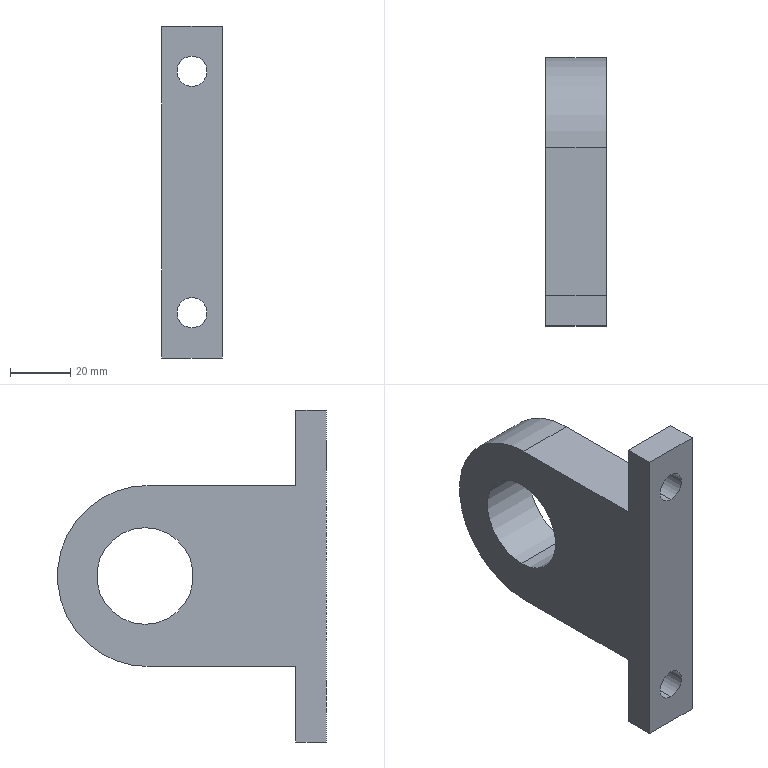Part | SolidWorks | features MoveFace 4, BaseBody 1, DelFace 1, HoleWzd 1, ICE 1, Split 1 | 1 solid | 16 faces | box 20 x 89 x 110 mm | volume 91419 mm3 | plane 9 | cylinder 7 | commonest cylinder face diameters 10 x4 32 x2 60 x1
STEP:
#1=CARTESIAN_POINT('',(-25.,46.,-25.));
#2=VERTEX_POINT('',#1);
#3=CARTESIAN_POINT('',(-25.,46.,-15.));
#4=VERTEX_POINT('',#3);
#5=CARTESIAN_POINT('',(-25.,46.,-20.));
#6=DIRECTION('',(0.,1.,0.));
#7=DIRECTION('',(-1.,0.,0.));
#8=AXIS2_PLACEMENT_3D('',#5,#6,#7);
#9=CIRCLE('',#8,5.);
#10=EDGE_CURVE('',#2,#4,#9,.T.);
#11=ORIENTED_EDGE('',*,*,#10,.F.);
#12=CARTESIAN_POINT('',(-25.,56.,-25.));
#13=VERTEX_POINT('',#12);
#14=CARTESIAN_POINT('',(-25.,10.,-25.));
#15=DIRECTION('',(0.,1.,0.));
#16=VECTOR('',#15,1000.);
#17=LINE('',#14,#16);
#18=EDGE_CURVE('',#2,#13,#17,.T.);
#19=ORIENTED_EDGE('',*,*,#18,.T.);
#20=CARTESIAN_POINT('',(-25.,56.,-15.));
#21=VERTEX_POINT('',#20);
#22=CARTESIAN_POINT('',(-25.,56.,-20.));
#23=DIRECTION('',(0.,1.,0.));
#24=DIRECTION('',(-1.,0.,0.));
#25=AXIS2_PLACEMENT_3D('',#22,#23,#24);
#26=CIRCLE('',#25,5.);
#27=EDGE_CURVE('',#13,#21,#26,.T.);
#28=ORIENTED_EDGE('',*,*,#27,.T.);
#29=CARTESIAN_POINT('',(-25.,10.,-15.));
#30=DIRECTION('',(0.,1.,0.));
#31=VECTOR('',#30,1000.);
#32=LINE('',#29,#31);
#33=EDGE_CURVE('',#4,#21,#32,.T.);
#34=ORIENTED_EDGE('',*,*,#33,.F.);
#35=EDGE_LOOP('',(#11,#19,#28,#34));
#36=FACE_OUTER_BOUND('',#35,.T.);
#37=CARTESIAN_POINT('',(-25.,10.,-20.));
#38=DIRECTION('',(0.,1.,0.));
#39=DIRECTION('',(0.,0.,1.));
#40=AXIS2_PLACEMENT_3D('',#37,#38,#39);
#41=CYLINDRICAL_SURFACE('',#40,5.);
#42=ADVANCED_FACE('',(#36),#41,.F.);
#43=CARTESIAN_POINT('',(-25.,46.,55.));
#44=VERTEX_POINT('',#43);
#45=CARTESIAN_POINT('',(-25.,46.,65.));
#46=VERTEX_POINT('',#45);
#47=CARTESIAN_POINT('',(-25.,46.,60.));
#48=DIRECTION('',(0.,1.,0.));
#49=DIRECTION('',(-1.,0.,0.));
#50=AXIS2_PLACEMENT_3D('',#47,#48,#49);
#51=CIRCLE('',#50,5.);
#52=EDGE_CURVE('',#44,#46,#51,.T.);
#53=ORIENTED_EDGE('',*,*,#52,.F.);
#54=CARTESIAN_POINT('',(-25.,56.,55.));
#55=VERTEX_POINT('',#54);
#56=CARTESIAN_POINT('',(-25.,10.,55.));
#57=DIRECTION('',(0.,1.,0.));
#58=VECTOR('',#57,1000.);
#59=LINE('',#56,#58);
#60=EDGE_CURVE('',#44,#55,#59,.T.);
#61=ORIENTED_EDGE('',*,*,#60,.T.);
#62=CARTESIAN_POINT('',(-25.,56.,65.));
#63=VERTEX_POINT('',#62);
#64=CARTESIAN_POINT('',(-25.,56.,60.));
#65=DIRECTION('',(0.,1.,0.));
#66=DIRECTION('',(-1.,0.,0.));
#67=AXIS2_PLACEMENT_3D('',#64,#65,#66);
#68=CIRCLE('',#67,5.);
#69=EDGE_CURVE('',#55,#63,#68,.T.);
#70=ORIENTED_EDGE('',*,*,#69,.T.);
#71=CARTESIAN_POINT('',(-25.,10.,65.));
#72=DIRECTION('',(0.,1.,0.));
#73=VECTOR('',#72,1000.);
#74=LINE('',#71,#73);
#75=EDGE_CURVE('',#46,#63,#74,.T.);
#76=ORIENTED_EDGE('',*,*,#75,.F.);
#77=EDGE_LOOP('',(#53,#61,#70,#76));
#78=FACE_OUTER_BOUND('',#77,.T.);
#79=CARTESIAN_POINT('',(-25.,10.,60.));
#80=DIRECTION('',(0.,1.,0.));
#81=DIRECTION('',(0.,0.,1.));
#82=AXIS2_PLACEMENT_3D('',#79,#80,#81);
#83=CYLINDRICAL_SURFACE('',#82,5.);
#84=ADVANCED_FACE('',(#78),#83,.F.);
#85=CARTESIAN_POINT('',(-35.,106.,36.));
#86=VERTEX_POINT('',#85);
#87=CARTESIAN_POINT('',(-35.,106.,4.));
#88=VERTEX_POINT('',#87);
#89=CARTESIAN_POINT('',(-35.,106.,20.));
#90=DIRECTION('',(1.,0.,0.));
#91=DIRECTION('',(0.,0.,-1.));
#92=AXIS2_PLACEMENT_3D('',#89,#90,#91);
#93=CIRCLE('',#92,16.);
#94=EDGE_CURVE('',#86,#88,#93,.T.);
#95=ORIENTED_EDGE('',*,*,#94,.F.);
#96=CARTESIAN_POINT('',(-15.,106.,36.));
#97=VERTEX_POINT('',#96);
#98=CARTESIAN_POINT('',(-35.,106.,36.));
#99=DIRECTION('',(1.,0.,0.));
#100=VECTOR('',#99,1000.);
#101=LINE('',#98,#100);
#102=EDGE_CURVE('',#86,#97,#101,.T.);
#103=ORIENTED_EDGE('',*,*,#102,.T.);
#104=CARTESIAN_POINT('',(-15.,106.,4.));
#105=VERTEX_POINT('',#104);
#106=CARTESIAN_POINT('',(-15.,106.,20.));
#107=DIRECTION('',(-1.,0.,0.));
#108=DIRECTION('',(0.,-1.,0.));
#109=AXIS2_PLACEMENT_3D('',#106,#107,#108);
#110=CIRCLE('',#109,16.);
#111=EDGE_CURVE('',#105,#97,#110,.T.);
#112=ORIENTED_EDGE('',*,*,#111,.F.);
#113=CARTESIAN_POINT('',(-35.,106.,4.));
#114=DIRECTION('',(1.,0.,0.));
#115=VECTOR('',#114,1000.);
#116=LINE('',#113,#115);
#117=EDGE_CURVE('',#88,#105,#116,.T.);
#118=ORIENTED_EDGE('',*,*,#117,.F.);
#119=EDGE_LOOP('',(#95,#103,#112,#118));
#120=FACE_OUTER_BOUND('',#119,.T.);
#121=CARTESIAN_POINT('',(-35.,106.,20.));
#122=DIRECTION('',(1.,0.,0.));
#123=DIRECTION('',(0.,0.,-1.));
#124=AXIS2_PLACEMENT_3D('',#121,#122,#123);
#125=CYLINDRICAL_SURFACE('',#124,16.);
#126=ADVANCED_FACE('',(#120),#125,.F.);
#127=CARTESIAN_POINT('',(-25.,46.,-20.));
#128=DIRECTION('',(0.,1.,0.));
#129=DIRECTION('',(-1.,0.,0.));
#130=AXIS2_PLACEMENT_3D('',#127,#128,#129);
#131=CIRCLE('',#130,5.);
#132=EDGE_CURVE('',#4,#2,#131,.T.);
#133=ORIENTED_EDGE('',*,*,#132,.T.);
#134=ORIENTED_EDGE('',*,*,#10,.T.);
#135=EDGE_LOOP('',(#133,#134));
#136=FACE_BOUND('',#135,.T.);
#137=CARTESIAN_POINT('',(-25.,46.,60.));
#138=DIRECTION('',(0.,1.,0.));
#139=DIRECTION('',(-1.,0.,0.));
#140=AXIS2_PLACEMENT_3D('',#137,#138,#139);
#141=CIRCLE('',#140,5.);
#142=EDGE_CURVE('',#46,#44,#141,.T.);
#143=ORIENTED_EDGE('',*,*,#142,.T.);
#144=ORIENTED_EDGE('',*,*,#52,.T.);
#145=EDGE_LOOP('',(#143,#144));
#146=FACE_BOUND('',#145,.T.);
#147=CARTESIAN_POINT('',(-15.,46.,75.));
#148=VERTEX_POINT('',#147);
#149=CARTESIAN_POINT('',(-15.,46.,-35.));
#150=VERTEX_POINT('',#149);
#151=CARTESIAN_POINT('',(-15.,46.,40.));
#152=DIRECTION('',(0.,0.,-1.));
#153=VECTOR('',#152,1000.);
#154=LINE('',#151,#153);
#155=EDGE_CURVE('',#148,#150,#154,.T.);
#156=ORIENTED_EDGE('',*,*,#155,.F.);
#157=CARTESIAN_POINT('',(-35.,46.,75.));
#158=VERTEX_POINT('',#157);
#159=CARTESIAN_POINT('',(-35.,46.,75.));
#160=DIRECTION('',(-1.,0.,0.));
#161=VECTOR('',#160,1000.);
#162=LINE('',#159,#161);
#163=EDGE_CURVE('',#148,#158,#162,.T.);
#164=ORIENTED_EDGE('',*,*,#163,.T.);
#165=CARTESIAN_POINT('',(-35.,46.,-35.));
#166=VERTEX_POINT('',#165);
#167=CARTESIAN_POINT('',(-35.,46.,40.));
#168=DIRECTION('',(0.,0.,-1.));
#169=VECTOR('',#168,1000.);
#170=LINE('',#167,#169);
#171=EDGE_CURVE('',#158,#166,#170,.T.);
#172=ORIENTED_EDGE('',*,*,#171,.T.);
#173=CARTESIAN_POINT('',(-35.,46.,-35.));
#174=DIRECTION('',(1.,0.,0.));
#175=VECTOR('',#174,1000.);
#176=LINE('',#173,#175);
#177=EDGE_CURVE('',#166,#150,#176,.T.);
#178=ORIENTED_EDGE('',*,*,#177,.T.);
#179=EDGE_LOOP('',(#156,#164,#172,#178));
#180=FACE_OUTER_BOUND('',#179,.T.);
#181=CARTESIAN_POINT('',(0.,46.,40.));
#182=DIRECTION('',(0.,1.,0.));
#183=DIRECTION('',(-1.,0.,0.));
#184=AXIS2_PLACEMENT_3D('',#181,#182,#183);
#185=PLANE('',#184);
#186=ADVANCED_FACE('',(#136,#146,#180),#185,.F.);
#187=CARTESIAN_POINT('',(-35.,105.,50.));
#188=VERTEX_POINT('',#187);
#189=CARTESIAN_POINT('',(-35.,56.,50.));
#190=VERTEX_POINT('',#189);
#191=CARTESIAN_POINT('',(-35.,0.,50.));
#192=DIRECTION('',(0.,-1.,0.));
#193=VECTOR('',#192,1000.);
#194=LINE('',#191,#193);
#195=EDGE_CURVE('',#188,#190,#194,.T.);
#196=ORIENTED_EDGE('',*,*,#195,.T.);
#197=CARTESIAN_POINT('',(-15.,56.,50.));
#198=VERTEX_POINT('',#197);
#199=CARTESIAN_POINT('',(0.,56.,50.));
#200=DIRECTION('',(1.,0.,0.));
#201=VECTOR('',#200,1000.);
#202=LINE('',#199,#201);
#203=EDGE_CURVE('',#190,#198,#202,.T.);
#204=ORIENTED_EDGE('',*,*,#203,.T.);
#205=CARTESIAN_POINT('',(-15.,105.,50.));
#206=VERTEX_POINT('',#205);
#207=CARTESIAN_POINT('',(-15.,125.,50.));
#208=DIRECTION('',(0.,-1.,0.));
#209=VECTOR('',#208,1000.);
#210=LINE('',#207,#209);
#211=EDGE_CURVE('',#206,#198,#210,.T.);
#212=ORIENTED_EDGE('',*,*,#211,.F.);
#213=CARTESIAN_POINT('',(0.,105.,50.));
#214=DIRECTION('',(1.,0.,0.));
#215=VECTOR('',#214,1000.);
#216=LINE('',#213,#215);
#217=EDGE_CURVE('',#188,#206,#216,.T.);
#218=ORIENTED_EDGE('',*,*,#217,.F.);
#219=EDGE_LOOP('',(#196,#204,#212,#218));
#220=FACE_OUTER_BOUND('',#219,.T.);
#221=CARTESIAN_POINT('',(0.,0.,50.));
#222=DIRECTION('',(0.,0.,-1.));
#223=DIRECTION('',(-1.,0.,0.));
#224=AXIS2_PLACEMENT_3D('',#221,#222,#223);
#225=PLANE('',#224);
#226=ADVANCED_FACE('',(#220),#225,.F.);
#227=CARTESIAN_POINT('',(-35.,56.,-10.));
#228=VERTEX_POINT('',#227);
#229=CARTESIAN_POINT('',(-35.,105.,-10.));
#230=VERTEX_POINT('',#229);
#231=CARTESIAN_POINT('',(-35.,0.,-10.));
#232=DIRECTION('',(0.,1.,0.));
#233=VECTOR('',#232,1000.);
#234=LINE('',#231,#233);
#235=EDGE_CURVE('',#228,#230,#234,.T.);
#236=ORIENTED_EDGE('',*,*,#235,.F.);
#237=CARTESIAN_POINT('',(-35.,56.,-35.));
#238=VERTEX_POINT('',#237);
#239=CARTESIAN_POINT('',(-35.,56.,0.));
#240=DIRECTION('',(0.,0.,-1.));
#241=VECTOR('',#240,1000.);
#242=LINE('',#239,#241);
#243=EDGE_CURVE('',#228,#238,#242,.T.);
#244=ORIENTED_EDGE('',*,*,#243,.T.);
#245=CARTESIAN_POINT('',(-35.,10.,-35.));
#246=DIRECTION('',(0.,-1.,0.));
#247=VECTOR('',#246,1000.);
#248=LINE('',#245,#247);
#249=EDGE_CURVE('',#238,#166,#248,.T.);
#250=ORIENTED_EDGE('',*,*,#249,.T.);
#251=ORIENTED_EDGE('',*,*,#171,.F.);
#252=CARTESIAN_POINT('',(-35.,56.,75.));
#253=VERTEX_POINT('',#252);
#254=CARTESIAN_POINT('',(-35.,10.,75.));
#255=DIRECTION('',(0.,-1.,0.));
#256=VECTOR('',#255,1000.);
#257=LINE('',#254,#256);
#258=EDGE_CURVE('',#253,#158,#257,.T.);
#259=ORIENTED_EDGE('',*,*,#258,.F.);
#260=CARTESIAN_POINT('',(-35.,56.,0.));
#261=DIRECTION('',(0.,0.,-1.));
#262=VECTOR('',#261,1000.);
#263=LINE('',#260,#262);
#264=EDGE_CURVE('',#253,#190,#263,.T.);
#265=ORIENTED_EDGE('',*,*,#264,.T.);
#266=ORIENTED_EDGE('',*,*,#195,.F.);
#267=CARTESIAN_POINT('',(-35.,105.,20.));
#268=DIRECTION('',(1.,0.,0.));
#269=DIRECTION('',(0.,0.,-1.));
#270=AXIS2_PLACEMENT_3D('',#267,#268,#269);
#271=CIRCLE('',#270,30.);
#272=EDGE_CURVE('',#230,#188,#271,.T.);
#273=ORIENTED_EDGE('',*,*,#272,.F.);
#274=EDGE_LOOP('',(#236,#244,#250,#251,#259,#265,#266,#273));
#275=FACE_OUTER_BOUND('',#274,.T.);
#276=CARTESIAN_POINT('',(-35.,106.,20.));
#277=DIRECTION('',(1.,0.,0.));
#278=DIRECTION('',(0.,0.,-1.));
#279=AXIS2_PLACEMENT_3D('',#276,#277,#278);
#280=CIRCLE('',#279,16.);
#281=EDGE_CURVE('',#88,#86,#280,.T.);
#282=ORIENTED_EDGE('',*,*,#281,.T.);
#283=ORIENTED_EDGE('',*,*,#94,.T.);
#284=EDGE_LOOP('',(#282,#283));
#285=FACE_BOUND('',#284,.T.);
#286=CARTESIAN_POINT('',(-35.,0.,40.));
#287=DIRECTION('',(1.,0.,0.));
#288=DIRECTION('',(0.,0.,-1.));
#289=AXIS2_PLACEMENT_3D('',#286,#287,#288);
#290=PLANE('',#289);
#291=ADVANCED_FACE('',(#275,#285),#290,.F.);
#292=ORIENTED_EDGE('',*,*,#102,.F.);
#293=ORIENTED_EDGE('',*,*,#281,.F.);
#294=ORIENTED_EDGE('',*,*,#117,.T.);
#295=CARTESIAN_POINT('',(-15.,106.,20.));
#296=DIRECTION('',(-1.,0.,0.));
#297=DIRECTION('',(0.,-1.,0.));
#298=AXIS2_PLACEMENT_3D('',#295,#296,#297);
#299=CIRCLE('',#298,16.);
#300=EDGE_CURVE('',#97,#105,#299,.T.);
#301=ORIENTED_EDGE('',*,*,#300,.F.);
#302=EDGE_LOOP('',(#292,#293,#294,#301));
#303=FACE_OUTER_BOUND('',#302,.T.);
#304=CARTESIAN_POINT('',(-35.,106.,20.));
#305=DIRECTION('',(1.,0.,0.));
#306=DIRECTION('',(0.,0.,-1.));
#307=AXIS2_PLACEMENT_3D('',#304,#305,#306);
#308=CYLINDRICAL_SURFACE('',#307,16.);
#309=ADVANCED_FACE('',(#303),#308,.F.);
#310=CARTESIAN_POINT('',(-15.,56.,-10.));
#311=VERTEX_POINT('',#310);
#312=CARTESIAN_POINT('',(0.,56.,-10.));
#313=DIRECTION('',(1.,0.,0.));
#314=VECTOR('',#313,1000.);
#315=LINE('',#312,#314);
#316=EDGE_CURVE('',#228,#311,#315,.T.);
#317=ORIENTED_EDGE('',*,*,#316,.F.);
#318=ORIENTED_EDGE('',*,*,#235,.T.);
#319=CARTESIAN_POINT('',(-15.,105.,-10.));
#320=VERTEX_POINT('',#319);
#321=CARTESIAN_POINT('',(0.,105.,-10.));
#322=DIRECTION('',(-1.,0.,0.));
#323=VECTOR('',#322,1000.);
#324=LINE('',#321,#323);
#325=EDGE_CURVE('',#320,#230,#324,.T.);
#326=ORIENTED_EDGE('',*,*,#325,.F.);
#327=CARTESIAN_POINT('',(-15.,125.,-10.));
#328=DIRECTION('',(0.,-1.,0.));
#329=VECTOR('',#328,1000.);
#330=LINE('',#327,#329);
#331=EDGE_CURVE('',#320,#311,#330,.T.);
#332=ORIENTED_EDGE('',*,*,#331,.T.);
#333=EDGE_LOOP('',(#317,#318,#326,#332));
#334=FACE_OUTER_BOUND('',#333,.T.);
#335=CARTESIAN_POINT('',(0.,0.,-10.));
#336=DIRECTION('',(0.,0.,-1.));
#337=DIRECTION('',(-1.,0.,0.));
#338=AXIS2_PLACEMENT_3D('',#335,#336,#337);
#339=PLANE('',#338);
#340=ADVANCED_FACE('',(#334),#339,.T.);
#341=CARTESIAN_POINT('',(-15.,105.,20.));
#342=DIRECTION('',(-1.,0.,0.));
#343=DIRECTION('',(0.,-1.,0.));
#344=AXIS2_PLACEMENT_3D('',#341,#342,#343);
#345=CIRCLE('',#344,30.);
#346=EDGE_CURVE('',#206,#320,#345,.T.);
#347=ORIENTED_EDGE('',*,*,#346,.T.);
#348=ORIENTED_EDGE('',*,*,#325,.T.);
#349=ORIENTED_EDGE('',*,*,#272,.T.);
#350=ORIENTED_EDGE('',*,*,#217,.T.);
#351=EDGE_LOOP('',(#347,#348,#349,#350));
#352=FACE_OUTER_BOUND('',#351,.T.);
#353=CARTESIAN_POINT('',(0.,105.,20.));
#354=DIRECTION('',(-1.,0.,0.));
#355=DIRECTION('',(0.,0.,1.));
#356=AXIS2_PLACEMENT_3D('',#353,#354,#355);
#357=CYLINDRICAL_SURFACE('',#356,30.);
#358=ADVANCED_FACE('',(#352),#357,.T.);
#359=ORIENTED_EDGE('',*,*,#211,.T.);
#360=CARTESIAN_POINT('',(-15.,56.,75.));
#361=VERTEX_POINT('',#360);
#362=CARTESIAN_POINT('',(-15.,56.,-10.));
#363=DIRECTION('',(0.,0.,1.));
#364=VECTOR('',#363,1000.);
#365=LINE('',#362,#364);
#366=EDGE_CURVE('',#198,#361,#365,.T.);
#367=ORIENTED_EDGE('',*,*,#366,.T.);
#368=CARTESIAN_POINT('',(-15.,10.,75.));
#369=DIRECTION('',(0.,-1.,0.));
#370=VECTOR('',#369,1000.);
#371=LINE('',#368,#370);
#372=EDGE_CURVE('',#361,#148,#371,.T.);
#373=ORIENTED_EDGE('',*,*,#372,.T.);
#374=ORIENTED_EDGE('',*,*,#155,.T.);
#375=CARTESIAN_POINT('',(-15.,56.,-35.));
#376=VERTEX_POINT('',#375);
#377=CARTESIAN_POINT('',(-15.,10.,-35.));
#378=DIRECTION('',(0.,-1.,0.));
#379=VECTOR('',#378,1000.);
#380=LINE('',#377,#379);
#381=EDGE_CURVE('',#376,#150,#380,.T.);
#382=ORIENTED_EDGE('',*,*,#381,.F.);
#383=CARTESIAN_POINT('',(-15.,56.,-10.));
#384=DIRECTION('',(0.,0.,1.));
#385=VECTOR('',#384,1000.);
#386=LINE('',#383,#385);
#387=EDGE_CURVE('',#376,#311,#386,.T.);
#388=ORIENTED_EDGE('',*,*,#387,.T.);
#389=ORIENTED_EDGE('',*,*,#331,.F.);
#390=ORIENTED_EDGE('',*,*,#346,.F.);
#391=EDGE_LOOP('',(#359,#367,#373,#374,#382,#388,#389,#390));
#392=FACE_OUTER_BOUND('',#391,.T.);
#393=ORIENTED_EDGE('',*,*,#111,.T.);
#394=ORIENTED_EDGE('',*,*,#300,.T.);
#395=EDGE_LOOP('',(#393,#394));
#396=FACE_BOUND('',#395,.T.);
#397=CARTESIAN_POINT('',(-15.,105.,-10.));
#398=DIRECTION('',(1.,0.,0.));
#399=DIRECTION('',(0.,1.,0.));
#400=AXIS2_PLACEMENT_3D('',#397,#398,#399);
#401=PLANE('',#400);
#402=ADVANCED_FACE('',(#392,#396),#401,.T.);
#403=ORIENTED_EDGE('',*,*,#177,.F.);
#404=ORIENTED_EDGE('',*,*,#249,.F.);
#405=CARTESIAN_POINT('',(-35.,56.,-35.));
#406=DIRECTION('',(1.,0.,0.));
#407=VECTOR('',#406,1000.);
#408=LINE('',#405,#407);
#409=EDGE_CURVE('',#238,#376,#408,.T.);
#410=ORIENTED_EDGE('',*,*,#409,.T.);
#411=ORIENTED_EDGE('',*,*,#381,.T.);
#412=EDGE_LOOP('',(#403,#404,#410,#411));
#413=FACE_OUTER_BOUND('',#412,.T.);
#414=CARTESIAN_POINT('',(-35.,10.,-35.));
#415=DIRECTION('',(0.,0.,-1.));
#416=DIRECTION('',(-1.,0.,0.));
#417=AXIS2_PLACEMENT_3D('',#414,#415,#416);
#418=PLANE('',#417);
#419=ADVANCED_FACE('',(#413),#418,.T.);
#420=CARTESIAN_POINT('',(-25.,56.,-20.));
#421=DIRECTION('',(0.,1.,0.));
#422=DIRECTION('',(-1.,0.,0.));
#423=AXIS2_PLACEMENT_3D('',#420,#421,#422);
#424=CIRCLE('',#423,5.);
#425=EDGE_CURVE('',#21,#13,#424,.T.);
#426=ORIENTED_EDGE('',*,*,#425,.F.);
#427=ORIENTED_EDGE('',*,*,#27,.F.);
#428=EDGE_LOOP('',(#426,#427));
#429=FACE_BOUND('',#428,.T.);
#430=ORIENTED_EDGE('',*,*,#243,.F.);
#431=ORIENTED_EDGE('',*,*,#316,.T.);
#432=ORIENTED_EDGE('',*,*,#387,.F.);
#433=ORIENTED_EDGE('',*,*,#409,.F.);
#434=EDGE_LOOP('',(#430,#431,#432,#433));
#435=FACE_OUTER_BOUND('',#434,.T.);
#436=CARTESIAN_POINT('',(0.,56.,0.));
#437=DIRECTION('',(0.,1.,0.));
#438=DIRECTION('',(-1.,0.,0.));
#439=AXIS2_PLACEMENT_3D('',#436,#437,#438);
#440=PLANE('',#439);
#441=ADVANCED_FACE('',(#429,#435),#440,.T.);
#442=CARTESIAN_POINT('',(-25.,56.,60.));
#443=DIRECTION('',(0.,1.,0.));
#444=DIRECTION('',(-1.,0.,0.));
#445=AXIS2_PLACEMENT_3D('',#442,#443,#444);
#446=CIRCLE('',#445,5.);
#447=EDGE_CURVE('',#63,#55,#446,.T.);
#448=ORIENTED_EDGE('',*,*,#447,.F.);
#449=ORIENTED_EDGE('',*,*,#69,.F.);
#450=EDGE_LOOP('',(#448,#449));
#451=FACE_BOUND('',#450,.T.);
#452=ORIENTED_EDGE('',*,*,#203,.F.);
#453=ORIENTED_EDGE('',*,*,#264,.F.);
#454=CARTESIAN_POINT('',(-35.,56.,75.));
#455=DIRECTION('',(-1.,0.,0.));
#456=VECTOR('',#455,1000.);
#457=LINE('',#454,#456);
#458=EDGE_CURVE('',#361,#253,#457,.T.);
#459=ORIENTED_EDGE('',*,*,#458,.F.);
#460=ORIENTED_EDGE('',*,*,#366,.F.);
#461=EDGE_LOOP('',(#452,#453,#459,#460));
#462=FACE_OUTER_BOUND('',#461,.T.);
#463=CARTESIAN_POINT('',(0.,56.,0.));
#464=DIRECTION('',(0.,1.,0.));
#465=DIRECTION('',(-1.,0.,0.));
#466=AXIS2_PLACEMENT_3D('',#463,#464,#465);
#467=PLANE('',#466);
#468=ADVANCED_FACE('',(#451,#462),#467,.T.);
#469=ORIENTED_EDGE('',*,*,#163,.F.);
#470=ORIENTED_EDGE('',*,*,#372,.F.);
#471=ORIENTED_EDGE('',*,*,#458,.T.);
#472=ORIENTED_EDGE('',*,*,#258,.T.);
#473=EDGE_LOOP('',(#469,#470,#471,#472));
#474=FACE_OUTER_BOUND('',#473,.T.);
#475=CARTESIAN_POINT('',(-35.,10.,75.));
#476=DIRECTION('',(0.,0.,1.));
#477=DIRECTION('',(1.,0.,0.));
#478=AXIS2_PLACEMENT_3D('',#475,#476,#477);
#479=PLANE('',#478);
#480=ADVANCED_FACE('',(#474),#479,.T.);
#481=ORIENTED_EDGE('',*,*,#60,.F.);
#482=ORIENTED_EDGE('',*,*,#142,.F.);
#483=ORIENTED_EDGE('',*,*,#75,.T.);
#484=ORIENTED_EDGE('',*,*,#447,.T.);
#485=EDGE_LOOP('',(#481,#482,#483,#484));
#486=FACE_OUTER_BOUND('',#485,.T.);
#487=CARTESIAN_POINT('',(-25.,10.,60.));
#488=DIRECTION('',(0.,1.,0.));
#489=DIRECTION('',(0.,0.,1.));
#490=AXIS2_PLACEMENT_3D('',#487,#488,#489);
#491=CYLINDRICAL_SURFACE('',#490,5.);
#492=ADVANCED_FACE('',(#486),#491,.F.);
#493=ORIENTED_EDGE('',*,*,#18,.F.);
#494=ORIENTED_EDGE('',*,*,#132,.F.);
#495=ORIENTED_EDGE('',*,*,#33,.T.);
#496=ORIENTED_EDGE('',*,*,#425,.T.);
#497=EDGE_LOOP('',(#493,#494,#495,#496));
#498=FACE_OUTER_BOUND('',#497,.T.);
#499=CARTESIAN_POINT('',(-25.,10.,-20.));
#500=DIRECTION('',(0.,1.,0.));
#501=DIRECTION('',(0.,0.,1.));
#502=AXIS2_PLACEMENT_3D('',#499,#500,#501);
#503=CYLINDRICAL_SURFACE('',#502,5.);
#504=ADVANCED_FACE('',(#498),#503,.F.);
#505=CLOSED_SHELL('',(#42,#84,#126,#186,#226,#291,#309,#340,#358,#402,#419,#441,#468,#480,#492,#504));
#506=MANIFOLD_SOLID_BREP('',#505);
#507=CARTESIAN_POINT('',(0.,0.,0.));
#508=DIRECTION('',(0.,0.,1.));
#509=DIRECTION('',(1.,0.,0.));
#510=AXIS2_PLACEMENT_3D('',#507,#508,#509);
#511=(LENGTH_UNIT()NAMED_UNIT(*)SI_UNIT(.MILLI.,.METRE.));
#512=UNCERTAINTY_MEASURE_WITH_UNIT(LENGTH_MEASURE(0.00001),#511,'','');
#513=(NAMED_UNIT(*)PLANE_ANGLE_UNIT()SI_UNIT($,.RADIAN.));
#514=(NAMED_UNIT(*)SI_UNIT($,.STERADIAN.)SOLID_ANGLE_UNIT());
#515=(GEOMETRIC_REPRESENTATION_CONTEXT(3)GLOBAL_UNCERTAINTY_ASSIGNED_CONTEXT((#512))GLOBAL_UNIT_ASSIGNED_CONTEXT((#511,#513,#514))REPRESENTATION_CONTEXT('',''));
#516=ADVANCED_BREP_SHAPE_REPRESENTATION('',(#506,#510),#515);